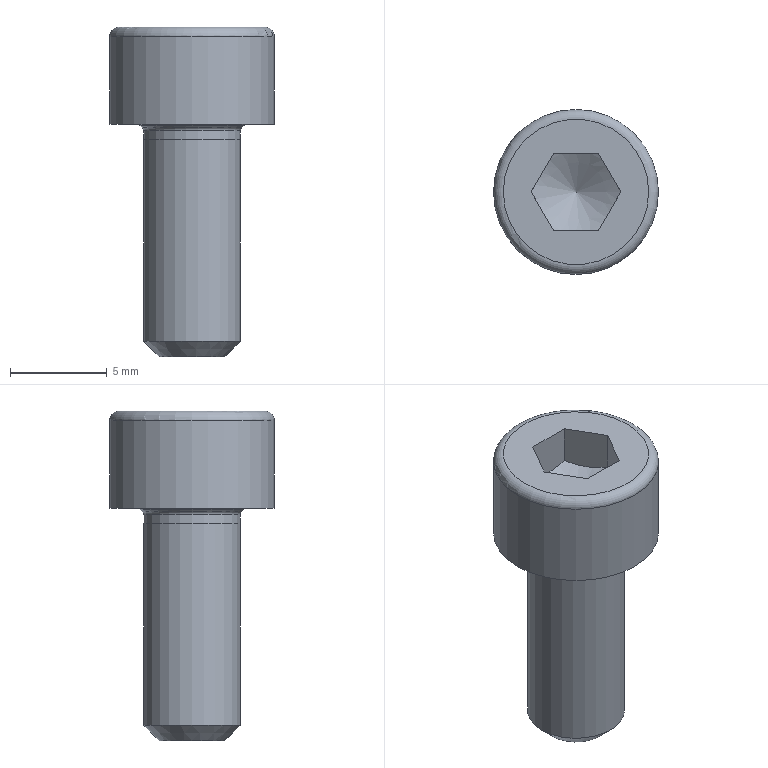Part | NX | features BREP 1, DATUM_CSYS 1 | 1 solid | 18 faces | box 8.5 x 8.5 x 17 mm | volume 479.07 mm3 | plane 9 | cone 3 | torus 3 | cylinder 3 | commonest cylinder face diameters 5 x2 8.5 x1
STEP:
#1=CARTESIAN_POINT('',(-2.309,0.,0.));
#2=VERTEX_POINT('',#1);
#3=CARTESIAN_POINT('',(-2.309,0.,-2.));
#4=VERTEX_POINT('',#3);
#5=CARTESIAN_POINT('',(-2.309,0.,0.));
#6=DIRECTION('',(0.,0.,-1.));
#7=VECTOR('',#6,1000.);
#8=LINE('',#5,#7);
#9=EDGE_CURVE('',#2,#4,#8,.T.);
#10=ORIENTED_EDGE('',*,*,#9,.T.);
#11=CARTESIAN_POINT('',(-1.155,2.,-2.));
#12=VERTEX_POINT('',#11);
#13=CARTESIAN_POINT('',(-2.309,0.,-2.));
#14=CARTESIAN_POINT('',(-1.732,1.,-2.333));
#15=CARTESIAN_POINT('',(-1.155,2.,-2.));
#16=(BOUNDED_CURVE()B_SPLINE_CURVE(2,(#13,#14,#15),.UNSPECIFIED.,.F.,.F.)B_SPLINE_CURVE_WITH_KNOTS((3,3),(0.,1.),.PIECEWISE_BEZIER_KNOTS.)CURVE()GEOMETRIC_REPRESENTATION_ITEM()RATIONAL_B_SPLINE_CURVE((1.,1.155,1.))REPRESENTATION_ITEM(''));
#17=EDGE_CURVE('',#4,#12,#16,.T.);
#18=ORIENTED_EDGE('',*,*,#17,.T.);
#19=CARTESIAN_POINT('',(-1.155,2.,0.));
#20=VERTEX_POINT('',#19);
#21=CARTESIAN_POINT('',(-1.155,2.,0.));
#22=DIRECTION('',(0.,0.,-1.));
#23=VECTOR('',#22,1000.);
#24=LINE('',#21,#23);
#25=EDGE_CURVE('',#20,#12,#24,.T.);
#26=ORIENTED_EDGE('',*,*,#25,.F.);
#27=CARTESIAN_POINT('',(-2.309,0.,0.));
#28=DIRECTION('',(0.5,0.866,0.));
#29=VECTOR('',#28,1000.);
#30=LINE('',#27,#29);
#31=EDGE_CURVE('',#2,#20,#30,.T.);
#32=ORIENTED_EDGE('',*,*,#31,.F.);
#33=EDGE_LOOP('',(#10,#18,#26,#32));
#34=FACE_BOUND('',#33,.T.);
#35=CARTESIAN_POINT('',(-1.732,1.,-1.25));
#36=DIRECTION('',(-0.866,0.5,0.));
#37=DIRECTION('',(-0.5,-0.866,0.));
#38=AXIS2_PLACEMENT_3D('',#35,#36,#37);
#39=PLANE('',#38);
#40=ADVANCED_FACE('',(#34),#39,.F.);
#41=ORIENTED_EDGE('',*,*,#25,.T.);
#42=CARTESIAN_POINT('',(1.155,2.,-2.));
#43=VERTEX_POINT('',#42);
#44=CARTESIAN_POINT('',(-1.155,2.,-2.));
#45=CARTESIAN_POINT('',(0.,2.,-2.333));
#46=CARTESIAN_POINT('',(1.155,2.,-2.));
#47=(BOUNDED_CURVE()B_SPLINE_CURVE(2,(#44,#45,#46),.UNSPECIFIED.,.F.,.F.)B_SPLINE_CURVE_WITH_KNOTS((3,3),(0.,1.),.PIECEWISE_BEZIER_KNOTS.)CURVE()GEOMETRIC_REPRESENTATION_ITEM()RATIONAL_B_SPLINE_CURVE((1.,1.155,1.))REPRESENTATION_ITEM(''));
#48=EDGE_CURVE('',#12,#43,#47,.T.);
#49=ORIENTED_EDGE('',*,*,#48,.T.);
#50=CARTESIAN_POINT('',(1.155,2.,0.));
#51=VERTEX_POINT('',#50);
#52=CARTESIAN_POINT('',(1.155,2.,0.));
#53=DIRECTION('',(0.,0.,-1.));
#54=VECTOR('',#53,1000.);
#55=LINE('',#52,#54);
#56=EDGE_CURVE('',#51,#43,#55,.T.);
#57=ORIENTED_EDGE('',*,*,#56,.F.);
#58=CARTESIAN_POINT('',(-1.155,2.,0.));
#59=DIRECTION('',(1.,0.,0.));
#60=VECTOR('',#59,1000.);
#61=LINE('',#58,#60);
#62=EDGE_CURVE('',#20,#51,#61,.T.);
#63=ORIENTED_EDGE('',*,*,#62,.F.);
#64=EDGE_LOOP('',(#41,#49,#57,#63));
#65=FACE_BOUND('',#64,.T.);
#66=CARTESIAN_POINT('',(0.,2.,-1.25));
#67=DIRECTION('',(0.,1.,0.));
#68=DIRECTION('',(-1.,0.,0.));
#69=AXIS2_PLACEMENT_3D('',#66,#67,#68);
#70=PLANE('',#69);
#71=ADVANCED_FACE('',(#65),#70,.F.);
#72=ORIENTED_EDGE('',*,*,#56,.T.);
#73=CARTESIAN_POINT('',(2.309,0.,-2.));
#74=VERTEX_POINT('',#73);
#75=CARTESIAN_POINT('',(1.155,2.,-2.));
#76=CARTESIAN_POINT('',(1.732,1.,-2.333));
#77=CARTESIAN_POINT('',(2.309,0.,-2.));
#78=(BOUNDED_CURVE()B_SPLINE_CURVE(2,(#75,#76,#77),.UNSPECIFIED.,.F.,.F.)B_SPLINE_CURVE_WITH_KNOTS((3,3),(0.,1.),.PIECEWISE_BEZIER_KNOTS.)CURVE()GEOMETRIC_REPRESENTATION_ITEM()RATIONAL_B_SPLINE_CURVE((1.,1.155,1.))REPRESENTATION_ITEM(''));
#79=EDGE_CURVE('',#43,#74,#78,.T.);
#80=ORIENTED_EDGE('',*,*,#79,.T.);
#81=CARTESIAN_POINT('',(2.309,0.,0.));
#82=VERTEX_POINT('',#81);
#83=CARTESIAN_POINT('',(2.309,0.,0.));
#84=DIRECTION('',(0.,0.,-1.));
#85=VECTOR('',#84,1000.);
#86=LINE('',#83,#85);
#87=EDGE_CURVE('',#82,#74,#86,.T.);
#88=ORIENTED_EDGE('',*,*,#87,.F.);
#89=CARTESIAN_POINT('',(1.155,2.,0.));
#90=DIRECTION('',(0.5,-0.866,0.));
#91=VECTOR('',#90,1000.);
#92=LINE('',#89,#91);
#93=EDGE_CURVE('',#51,#82,#92,.T.);
#94=ORIENTED_EDGE('',*,*,#93,.F.);
#95=EDGE_LOOP('',(#72,#80,#88,#94));
#96=FACE_BOUND('',#95,.T.);
#97=CARTESIAN_POINT('',(1.732,1.,-1.25));
#98=DIRECTION('',(0.866,0.5,0.));
#99=DIRECTION('',(-0.5,0.866,0.));
#100=AXIS2_PLACEMENT_3D('',#97,#98,#99);
#101=PLANE('',#100);
#102=ADVANCED_FACE('',(#96),#101,.F.);
#103=ORIENTED_EDGE('',*,*,#87,.T.);
#104=CARTESIAN_POINT('',(1.155,-2.,-2.));
#105=VERTEX_POINT('',#104);
#106=CARTESIAN_POINT('',(2.309,0.,-2.));
#107=CARTESIAN_POINT('',(1.732,-1.,-2.333));
#108=CARTESIAN_POINT('',(1.155,-2.,-2.));
#109=(BOUNDED_CURVE()B_SPLINE_CURVE(2,(#106,#107,#108),.UNSPECIFIED.,.F.,.F.)B_SPLINE_CURVE_WITH_KNOTS((3,3),(0.,1.),.PIECEWISE_BEZIER_KNOTS.)CURVE()GEOMETRIC_REPRESENTATION_ITEM()RATIONAL_B_SPLINE_CURVE((1.,1.155,1.))REPRESENTATION_ITEM(''));
#110=EDGE_CURVE('',#74,#105,#109,.T.);
#111=ORIENTED_EDGE('',*,*,#110,.T.);
#112=CARTESIAN_POINT('',(1.155,-2.,0.));
#113=VERTEX_POINT('',#112);
#114=CARTESIAN_POINT('',(1.155,-2.,0.));
#115=DIRECTION('',(0.,0.,-1.));
#116=VECTOR('',#115,1000.);
#117=LINE('',#114,#116);
#118=EDGE_CURVE('',#113,#105,#117,.T.);
#119=ORIENTED_EDGE('',*,*,#118,.F.);
#120=CARTESIAN_POINT('',(2.309,0.,0.));
#121=DIRECTION('',(-0.5,-0.866,0.));
#122=VECTOR('',#121,1000.);
#123=LINE('',#120,#122);
#124=EDGE_CURVE('',#82,#113,#123,.T.);
#125=ORIENTED_EDGE('',*,*,#124,.F.);
#126=EDGE_LOOP('',(#103,#111,#119,#125));
#127=FACE_BOUND('',#126,.T.);
#128=CARTESIAN_POINT('',(1.732,-1.,-1.25));
#129=DIRECTION('',(0.866,-0.5,0.));
#130=DIRECTION('',(0.5,0.866,0.));
#131=AXIS2_PLACEMENT_3D('',#128,#129,#130);
#132=PLANE('',#131);
#133=ADVANCED_FACE('',(#127),#132,.F.);
#134=ORIENTED_EDGE('',*,*,#118,.T.);
#135=CARTESIAN_POINT('',(-1.155,-2.,-2.));
#136=VERTEX_POINT('',#135);
#137=CARTESIAN_POINT('',(1.155,-2.,-2.));
#138=CARTESIAN_POINT('',(0.,-2.,-2.333));
#139=CARTESIAN_POINT('',(-1.155,-2.,-2.));
#140=(BOUNDED_CURVE()B_SPLINE_CURVE(2,(#137,#138,#139),.UNSPECIFIED.,.F.,.F.)B_SPLINE_CURVE_WITH_KNOTS((3,3),(0.,1.),.PIECEWISE_BEZIER_KNOTS.)CURVE()GEOMETRIC_REPRESENTATION_ITEM()RATIONAL_B_SPLINE_CURVE((1.,1.155,1.))REPRESENTATION_ITEM(''));
#141=EDGE_CURVE('',#105,#136,#140,.T.);
#142=ORIENTED_EDGE('',*,*,#141,.T.);
#143=CARTESIAN_POINT('',(-1.155,-2.,0.));
#144=VERTEX_POINT('',#143);
#145=CARTESIAN_POINT('',(-1.155,-2.,0.));
#146=DIRECTION('',(0.,0.,-1.));
#147=VECTOR('',#146,1000.);
#148=LINE('',#145,#147);
#149=EDGE_CURVE('',#144,#136,#148,.T.);
#150=ORIENTED_EDGE('',*,*,#149,.F.);
#151=CARTESIAN_POINT('',(1.155,-2.,0.));
#152=DIRECTION('',(-1.,0.,0.));
#153=VECTOR('',#152,1000.);
#154=LINE('',#151,#153);
#155=EDGE_CURVE('',#113,#144,#154,.T.);
#156=ORIENTED_EDGE('',*,*,#155,.F.);
#157=EDGE_LOOP('',(#134,#142,#150,#156));
#158=FACE_BOUND('',#157,.T.);
#159=CARTESIAN_POINT('',(0.,-2.,-1.25));
#160=DIRECTION('',(0.,-1.,0.));
#161=DIRECTION('',(1.,0.,0.));
#162=AXIS2_PLACEMENT_3D('',#159,#160,#161);
#163=PLANE('',#162);
#164=ADVANCED_FACE('',(#158),#163,.F.);
#165=ORIENTED_EDGE('',*,*,#149,.T.);
#166=CARTESIAN_POINT('',(-1.155,-2.,-2.));
#167=CARTESIAN_POINT('',(-1.732,-1.,-2.333));
#168=CARTESIAN_POINT('',(-2.309,0.,-2.));
#169=(BOUNDED_CURVE()B_SPLINE_CURVE(2,(#166,#167,#168),.UNSPECIFIED.,.F.,.F.)B_SPLINE_CURVE_WITH_KNOTS((3,3),(0.,1.),.PIECEWISE_BEZIER_KNOTS.)CURVE()GEOMETRIC_REPRESENTATION_ITEM()RATIONAL_B_SPLINE_CURVE((1.,1.155,1.))REPRESENTATION_ITEM(''));
#170=EDGE_CURVE('',#136,#4,#169,.T.);
#171=ORIENTED_EDGE('',*,*,#170,.T.);
#172=ORIENTED_EDGE('',*,*,#9,.F.);
#173=CARTESIAN_POINT('',(-1.155,-2.,0.));
#174=DIRECTION('',(-0.5,0.866,0.));
#175=VECTOR('',#174,1000.);
#176=LINE('',#173,#175);
#177=EDGE_CURVE('',#144,#2,#176,.T.);
#178=ORIENTED_EDGE('',*,*,#177,.F.);
#179=EDGE_LOOP('',(#165,#171,#172,#178));
#180=FACE_BOUND('',#179,.T.);
#181=CARTESIAN_POINT('',(-1.732,-1.,-1.25));
#182=DIRECTION('',(-0.866,-0.5,0.));
#183=DIRECTION('',(0.5,-0.866,0.));
#184=AXIS2_PLACEMENT_3D('',#181,#182,#183);
#185=PLANE('',#184);
#186=ADVANCED_FACE('',(#180),#185,.F.);
#187=ORIENTED_EDGE('',*,*,#79,.F.);
#188=ORIENTED_EDGE('',*,*,#48,.F.);
#189=ORIENTED_EDGE('',*,*,#17,.F.);
#190=ORIENTED_EDGE('',*,*,#170,.F.);
#191=ORIENTED_EDGE('',*,*,#141,.F.);
#192=ORIENTED_EDGE('',*,*,#110,.F.);
#193=CARTESIAN_POINT('',(0.,0.,-3.333));
#194=VERTEX_POINT('',#193);
#195=CARTESIAN_POINT('',(2.309,0.,-2.));
#196=DIRECTION('',(-0.866,0.,-0.5));
#197=VECTOR('',#196,1000.);
#198=LINE('',#195,#197);
#199=EDGE_CURVE('',#74,#194,#198,.T.);
#200=ORIENTED_EDGE('',*,*,#199,.T.);
#201=ORIENTED_EDGE('',*,*,#199,.F.);
#202=EDGE_LOOP('',(#187,#188,#189,#190,#191,#192,#200,#201));
#203=FACE_BOUND('',#202,.T.);
#204=CARTESIAN_POINT('',(0.,0.,-3.333));
#205=DIRECTION('',(0.,0.,1.));
#206=DIRECTION('',(-1.,0.,0.));
#207=AXIS2_PLACEMENT_3D('',#204,#205,#206);
#208=CONICAL_SURFACE('',#207,0.,1.047);
#209=ADVANCED_FACE('',(#203),#208,.F.);
#210=CARTESIAN_POINT('',(3.75,0.,0.));
#211=VERTEX_POINT('',#210);
#212=CARTESIAN_POINT('',(0.,0.,0.));
#213=DIRECTION('',(0.,0.,-1.));
#214=DIRECTION('',(1.,0.,0.));
#215=AXIS2_PLACEMENT_3D('',#212,#213,#214);
#216=CIRCLE('',#215,3.75);
#217=EDGE_CURVE('',#211,#211,#216,.T.);
#218=ORIENTED_EDGE('',*,*,#217,.F.);
#219=EDGE_LOOP('',(#218));
#220=FACE_BOUND('',#219,.T.);
#221=ORIENTED_EDGE('',*,*,#124,.T.);
#222=ORIENTED_EDGE('',*,*,#155,.T.);
#223=ORIENTED_EDGE('',*,*,#177,.T.);
#224=ORIENTED_EDGE('',*,*,#31,.T.);
#225=ORIENTED_EDGE('',*,*,#62,.T.);
#226=ORIENTED_EDGE('',*,*,#93,.T.);
#227=EDGE_LOOP('',(#221,#222,#223,#224,#225,#226));
#228=FACE_BOUND('',#227,.T.);
#229=CARTESIAN_POINT('',(0.,0.,0.));
#230=DIRECTION('',(0.,0.,-1.));
#231=DIRECTION('',(-1.,0.,0.));
#232=AXIS2_PLACEMENT_3D('',#229,#230,#231);
#233=PLANE('',#232);
#234=ADVANCED_FACE('',(#220,#228),#233,.F.);
#235=CARTESIAN_POINT('',(4.25,0.,-0.5));
#236=VERTEX_POINT('',#235);
#237=CARTESIAN_POINT('',(3.75,0.,-0.5));
#238=DIRECTION('',(0.,-1.,0.));
#239=DIRECTION('',(1.,0.,0.));
#240=AXIS2_PLACEMENT_3D('',#237,#238,#239);
#241=CIRCLE('',#240,0.5);
#242=EDGE_CURVE('',#236,#211,#241,.T.);
#243=ORIENTED_EDGE('',*,*,#242,.F.);
#244=CARTESIAN_POINT('',(0.,0.,-0.5));
#245=DIRECTION('',(0.,0.,-1.));
#246=DIRECTION('',(1.,0.,0.));
#247=AXIS2_PLACEMENT_3D('',#244,#245,#246);
#248=CIRCLE('',#247,4.25);
#249=EDGE_CURVE('',#236,#236,#248,.T.);
#250=ORIENTED_EDGE('',*,*,#249,.F.);
#251=ORIENTED_EDGE('',*,*,#242,.T.);
#252=ORIENTED_EDGE('',*,*,#217,.T.);
#253=EDGE_LOOP('',(#243,#250,#251,#252));
#254=FACE_BOUND('',#253,.T.);
#255=CARTESIAN_POINT('',(0.,0.,-0.5));
#256=DIRECTION('',(0.,0.,1.));
#257=DIRECTION('',(-1.,0.,0.));
#258=AXIS2_PLACEMENT_3D('',#255,#256,#257);
#259=TOROIDAL_SURFACE('',#258,3.75,0.5);
#260=ADVANCED_FACE('',(#254),#259,.T.);
#261=CARTESIAN_POINT('',(4.25,0.,-5.));
#262=VERTEX_POINT('',#261);
#263=CARTESIAN_POINT('',(0.,0.,-5.));
#264=DIRECTION('',(0.,0.,1.));
#265=DIRECTION('',(1.,0.,0.));
#266=AXIS2_PLACEMENT_3D('',#263,#264,#265);
#267=CIRCLE('',#266,4.25);
#268=EDGE_CURVE('',#262,#262,#267,.T.);
#269=ORIENTED_EDGE('',*,*,#268,.T.);
#270=CARTESIAN_POINT('',(4.25,0.,-5.));
#271=DIRECTION('',(0.,0.,1.));
#272=VECTOR('',#271,1000.);
#273=LINE('',#270,#272);
#274=EDGE_CURVE('',#262,#236,#273,.T.);
#275=ORIENTED_EDGE('',*,*,#274,.T.);
#276=ORIENTED_EDGE('',*,*,#249,.T.);
#277=ORIENTED_EDGE('',*,*,#274,.F.);
#278=EDGE_LOOP('',(#269,#275,#276,#277));
#279=FACE_BOUND('',#278,.T.);
#280=CARTESIAN_POINT('',(0.,0.,-5.));
#281=DIRECTION('',(0.,0.,1.));
#282=DIRECTION('',(-1.,0.,0.));
#283=AXIS2_PLACEMENT_3D('',#280,#281,#282);
#284=CYLINDRICAL_SURFACE('',#283,4.25);
#285=ADVANCED_FACE('',(#279),#284,.T.);
#286=ORIENTED_EDGE('',*,*,#268,.F.);
#287=EDGE_LOOP('',(#286));
#288=FACE_BOUND('',#287,.T.);
#289=CARTESIAN_POINT('',(2.84,0.,-5.));
#290=VERTEX_POINT('',#289);
#291=CARTESIAN_POINT('',(0.,0.,-5.));
#292=DIRECTION('',(0.,0.,1.));
#293=DIRECTION('',(1.,0.,0.));
#294=AXIS2_PLACEMENT_3D('',#291,#292,#293);
#295=CIRCLE('',#294,2.84);
#296=EDGE_CURVE('',#290,#290,#295,.T.);
#297=ORIENTED_EDGE('',*,*,#296,.T.);
#298=EDGE_LOOP('',(#297));
#299=FACE_BOUND('',#298,.T.);
#300=CARTESIAN_POINT('',(0.,0.,-5.));
#301=DIRECTION('',(0.,0.,1.));
#302=DIRECTION('',(-1.,0.,0.));
#303=AXIS2_PLACEMENT_3D('',#300,#301,#302);
#304=PLANE('',#303);
#305=ADVANCED_FACE('',(#288,#299),#304,.F.);
#306=CARTESIAN_POINT('',(2.699,0.,-5.059));
#307=VERTEX_POINT('',#306);
#308=CARTESIAN_POINT('',(0.,0.,-5.059));
#309=DIRECTION('',(0.,0.,1.));
#310=DIRECTION('',(1.,0.,0.));
#311=AXIS2_PLACEMENT_3D('',#308,#309,#310);
#312=CIRCLE('',#311,2.699);
#313=EDGE_CURVE('',#307,#307,#312,.T.);
#314=ORIENTED_EDGE('',*,*,#313,.T.);
#315=CARTESIAN_POINT('',(2.84,0.,-5.2));
#316=DIRECTION('',(0.,1.,0.));
#317=DIRECTION('',(-0.7071,0.,0.7071));
#318=AXIS2_PLACEMENT_3D('',#315,#316,#317);
#319=CIRCLE('',#318,0.2);
#320=EDGE_CURVE('',#307,#290,#319,.T.);
#321=ORIENTED_EDGE('',*,*,#320,.T.);
#322=ORIENTED_EDGE('',*,*,#296,.F.);
#323=ORIENTED_EDGE('',*,*,#320,.F.);
#324=EDGE_LOOP('',(#314,#321,#322,#323));
#325=FACE_BOUND('',#324,.T.);
#326=CARTESIAN_POINT('',(0.,0.,-5.2));
#327=DIRECTION('',(0.,0.,-1.));
#328=DIRECTION('',(-1.,0.,0.));
#329=AXIS2_PLACEMENT_3D('',#326,#327,#328);
#330=TOROIDAL_SURFACE('',#329,2.84,0.2);
#331=ADVANCED_FACE('',(#325),#330,.F.);
#332=CARTESIAN_POINT('',(2.559,0.,-5.199));
#333=VERTEX_POINT('',#332);
#334=CARTESIAN_POINT('',(0.,0.,-5.199));
#335=DIRECTION('',(0.,0.,1.));
#336=DIRECTION('',(1.,0.,0.));
#337=AXIS2_PLACEMENT_3D('',#334,#335,#336);
#338=CIRCLE('',#337,2.559);
#339=EDGE_CURVE('',#333,#333,#338,.T.);
#340=ORIENTED_EDGE('',*,*,#339,.T.);
#341=CARTESIAN_POINT('',(2.559,0.,-5.199));
#342=DIRECTION('',(0.7071,0.,0.7071));
#343=VECTOR('',#342,1000.);
#344=LINE('',#341,#343);
#345=EDGE_CURVE('',#333,#307,#344,.T.);
#346=ORIENTED_EDGE('',*,*,#345,.T.);
#347=ORIENTED_EDGE('',*,*,#313,.F.);
#348=ORIENTED_EDGE('',*,*,#345,.F.);
#349=EDGE_LOOP('',(#340,#346,#347,#348));
#350=FACE_BOUND('',#349,.T.);
#351=CARTESIAN_POINT('',(0.,0.,-5.199));
#352=DIRECTION('',(0.,0.,1.));
#353=DIRECTION('',(-1.,0.,0.));
#354=AXIS2_PLACEMENT_3D('',#351,#352,#353);
#355=CONICAL_SURFACE('',#354,2.559,0.7854);
#356=ADVANCED_FACE('',(#350),#355,.T.);
#357=CARTESIAN_POINT('',(2.5,0.,-5.34));
#358=VERTEX_POINT('',#357);
#359=CARTESIAN_POINT('',(0.,0.,-5.34));
#360=DIRECTION('',(0.,0.,1.));
#361=DIRECTION('',(1.,0.,0.));
#362=AXIS2_PLACEMENT_3D('',#359,#360,#361);
#363=CIRCLE('',#362,2.5);
#364=EDGE_CURVE('',#358,#358,#363,.T.);
#365=ORIENTED_EDGE('',*,*,#364,.T.);
#366=CARTESIAN_POINT('',(2.7,0.,-5.34));
#367=DIRECTION('',(0.,1.,0.));
#368=DIRECTION('',(-1.,0.,0.));
#369=AXIS2_PLACEMENT_3D('',#366,#367,#368);
#370=CIRCLE('',#369,0.2);
#371=EDGE_CURVE('',#358,#333,#370,.T.);
#372=ORIENTED_EDGE('',*,*,#371,.T.);
#373=ORIENTED_EDGE('',*,*,#339,.F.);
#374=ORIENTED_EDGE('',*,*,#371,.F.);
#375=EDGE_LOOP('',(#365,#372,#373,#374));
#376=FACE_BOUND('',#375,.T.);
#377=CARTESIAN_POINT('',(0.,0.,-5.34));
#378=DIRECTION('',(0.,0.,-1.));
#379=DIRECTION('',(-1.,0.,0.));
#380=AXIS2_PLACEMENT_3D('',#377,#378,#379);
#381=TOROIDAL_SURFACE('',#380,2.7,0.2);
#382=ADVANCED_FACE('',(#376),#381,.F.);
#383=CARTESIAN_POINT('',(2.5,0.,-5.8));
#384=VERTEX_POINT('',#383);
#385=CARTESIAN_POINT('',(0.,0.,-5.8));
#386=DIRECTION('',(0.,0.,1.));
#387=DIRECTION('',(1.,0.,0.));
#388=AXIS2_PLACEMENT_3D('',#385,#386,#387);
#389=CIRCLE('',#388,2.5);
#390=EDGE_CURVE('',#384,#384,#389,.T.);
#391=ORIENTED_EDGE('',*,*,#390,.T.);
#392=CARTESIAN_POINT('',(2.5,0.,-5.8));
#393=DIRECTION('',(0.,0.,1.));
#394=VECTOR('',#393,1000.);
#395=LINE('',#392,#394);
#396=EDGE_CURVE('',#384,#358,#395,.T.);
#397=ORIENTED_EDGE('',*,*,#396,.T.);
#398=ORIENTED_EDGE('',*,*,#364,.F.);
#399=ORIENTED_EDGE('',*,*,#396,.F.);
#400=EDGE_LOOP('',(#391,#397,#398,#399));
#401=FACE_BOUND('',#400,.T.);
#402=CARTESIAN_POINT('',(0.,0.,-5.8));
#403=DIRECTION('',(0.,0.,1.));
#404=DIRECTION('',(-1.,0.,0.));
#405=AXIS2_PLACEMENT_3D('',#402,#403,#404);
#406=CYLINDRICAL_SURFACE('',#405,2.5);
#407=ADVANCED_FACE('',(#401),#406,.T.);
#408=ORIENTED_EDGE('',*,*,#390,.F.);
#409=CARTESIAN_POINT('',(2.5,0.,-16.2));
#410=VERTEX_POINT('',#409);
#411=CARTESIAN_POINT('',(2.5,0.,-16.2));
#412=DIRECTION('',(0.,0.,1.));
#413=VECTOR('',#412,1000.);
#414=LINE('',#411,#413);
#415=EDGE_CURVE('',#410,#384,#414,.T.);
#416=ORIENTED_EDGE('',*,*,#415,.F.);
#417=CARTESIAN_POINT('',(0.,0.,-16.2));
#418=DIRECTION('',(0.,0.,-1.));
#419=DIRECTION('',(1.,0.,0.));
#420=AXIS2_PLACEMENT_3D('',#417,#418,#419);
#421=CIRCLE('',#420,2.5);
#422=EDGE_CURVE('',#410,#410,#421,.T.);
#423=ORIENTED_EDGE('',*,*,#422,.F.);
#424=ORIENTED_EDGE('',*,*,#415,.T.);
#425=EDGE_LOOP('',(#408,#416,#423,#424));
#426=FACE_BOUND('',#425,.T.);
#427=CARTESIAN_POINT('',(0.,0.,-17.));
#428=DIRECTION('',(0.,0.,1.));
#429=DIRECTION('',(-1.,0.,0.));
#430=AXIS2_PLACEMENT_3D('',#427,#428,#429);
#431=CYLINDRICAL_SURFACE('',#430,2.5);
#432=ADVANCED_FACE('',(#426),#431,.T.);
#433=CARTESIAN_POINT('',(1.7,0.,-17.));
#434=VERTEX_POINT('',#433);
#435=CARTESIAN_POINT('',(0.,0.,-17.));
#436=DIRECTION('',(0.,0.,-1.));
#437=DIRECTION('',(1.,0.,0.));
#438=AXIS2_PLACEMENT_3D('',#435,#436,#437);
#439=CIRCLE('',#438,1.7);
#440=EDGE_CURVE('',#434,#434,#439,.T.);
#441=ORIENTED_EDGE('',*,*,#440,.T.);
#442=EDGE_LOOP('',(#441));
#443=FACE_BOUND('',#442,.T.);
#444=CARTESIAN_POINT('',(0.,0.,-17.));
#445=DIRECTION('',(0.,0.,1.));
#446=DIRECTION('',(-1.,0.,0.));
#447=AXIS2_PLACEMENT_3D('',#444,#445,#446);
#448=PLANE('',#447);
#449=ADVANCED_FACE('',(#443),#448,.F.);
#450=ORIENTED_EDGE('',*,*,#440,.F.);
#451=CARTESIAN_POINT('',(1.7,0.,-17.));
#452=DIRECTION('',(0.7071,0.,0.7071));
#453=VECTOR('',#452,1000.);
#454=LINE('',#451,#453);
#455=EDGE_CURVE('',#434,#410,#454,.T.);
#456=ORIENTED_EDGE('',*,*,#455,.T.);
#457=ORIENTED_EDGE('',*,*,#422,.T.);
#458=ORIENTED_EDGE('',*,*,#455,.F.);
#459=EDGE_LOOP('',(#450,#456,#457,#458));
#460=FACE_BOUND('',#459,.T.);
#461=CARTESIAN_POINT('',(0.,0.,-17.));
#462=DIRECTION('',(0.,0.,1.));
#463=DIRECTION('',(-1.,0.,0.));
#464=AXIS2_PLACEMENT_3D('',#461,#462,#463);
#465=CONICAL_SURFACE('',#464,1.7,0.7854);
#466=ADVANCED_FACE('',(#460),#465,.T.);
#467=CLOSED_SHELL('',(#40,#71,#102,#133,#164,#186,#209,#234,#260,#285,#305,#331,#356,#382,#407,#432,#449,#466));
#468=MANIFOLD_SOLID_BREP('',#467);
#469=(LENGTH_UNIT()NAMED_UNIT(*)SI_UNIT(.MILLI.,.METRE.));
#470=UNCERTAINTY_MEASURE_WITH_UNIT(LENGTH_MEASURE(0.00001),#469,'','');
#471=(NAMED_UNIT(*)PLANE_ANGLE_UNIT()SI_UNIT($,.RADIAN.));
#472=(NAMED_UNIT(*)SI_UNIT($,.STERADIAN.)SOLID_ANGLE_UNIT());
#473=(GEOMETRIC_REPRESENTATION_CONTEXT(3)GLOBAL_UNCERTAINTY_ASSIGNED_CONTEXT((#470))GLOBAL_UNIT_ASSIGNED_CONTEXT((#469,#471,#472))REPRESENTATION_CONTEXT('',''));
#474=ADVANCED_BREP_SHAPE_REPRESENTATION('',(#468),#473);